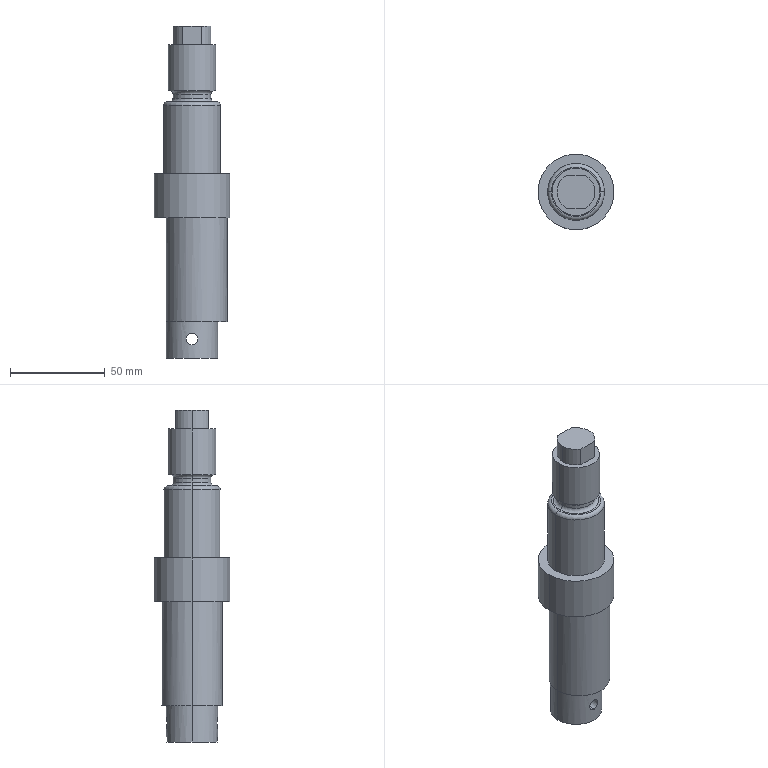Part | SolidWorks | features Boss 6, Chamfer 2, Cut 2, Extrusion 1, Fillet 1 | 1 solid | 33 faces | box 40 x 40 x 175 mm | volume 126777 mm3 | cylinder 17 | plane 10 | torus 6 | commonest cylinder face diameters 20 x5 6 x2 25 x2 27 x2 30 x2 32 x2
STEP:
#1=CARTESIAN_POINT('',(-12.,0.,141.));
#2=VERTEX_POINT('',#1);
#3=CARTESIAN_POINT('',(12.,0.,141.));
#4=VERTEX_POINT('',#3);
#5=CARTESIAN_POINT('',(0.,0.,141.));
#6=DIRECTION('',(0.,0.,1.));
#7=DIRECTION('',(1.,0.,0.));
#8=AXIS2_PLACEMENT_3D('',#5,#6,#7);
#9=CIRCLE('',#8,12.);
#10=EDGE_CURVE('',#2,#4,#9,.T.);
#11=ORIENTED_EDGE('',*,*,#10,.F.);
#12=CARTESIAN_POINT('',(-10.,0.,139.));
#13=VERTEX_POINT('',#12);
#14=CARTESIAN_POINT('',(-12.,0.,139.));
#15=DIRECTION('',(0.,1.,0.));
#16=DIRECTION('',(-1.,0.,0.));
#17=AXIS2_PLACEMENT_3D('',#14,#15,#16);
#18=CIRCLE('',#17,2.);
#19=EDGE_CURVE('',#2,#13,#18,.T.);
#20=ORIENTED_EDGE('',*,*,#19,.T.);
#21=CARTESIAN_POINT('',(10.,0.,139.));
#22=VERTEX_POINT('',#21);
#23=CARTESIAN_POINT('',(0.,0.,139.));
#24=DIRECTION('',(0.,0.,-1.));
#25=DIRECTION('',(1.,0.,0.));
#26=AXIS2_PLACEMENT_3D('',#23,#24,#25);
#27=CIRCLE('',#26,10.);
#28=EDGE_CURVE('',#22,#13,#27,.T.);
#29=ORIENTED_EDGE('',*,*,#28,.F.);
#30=CARTESIAN_POINT('',(12.,0.,139.));
#31=DIRECTION('',(0.,-1.,0.));
#32=DIRECTION('',(0.,0.,-1.));
#33=AXIS2_PLACEMENT_3D('',#30,#31,#32);
#34=CIRCLE('',#33,2.);
#35=EDGE_CURVE('',#4,#22,#34,.T.);
#36=ORIENTED_EDGE('',*,*,#35,.F.);
#37=EDGE_LOOP('',(#11,#20,#29,#36));
#38=FACE_OUTER_BOUND('',#37,.T.);
#39=CARTESIAN_POINT('',(0.,0.,139.));
#40=DIRECTION('',(0.,0.,1.));
#41=DIRECTION('',(1.,0.,0.));
#42=AXIS2_PLACEMENT_3D('',#39,#40,#41);
#43=TOROIDAL_SURFACE('',#42,12.,2.);
#44=ADVANCED_FACE('',(#38),#43,.F.);
#45=CARTESIAN_POINT('',(-15.,0.,133.));
#46=VERTEX_POINT('',#45);
#47=CARTESIAN_POINT('',(15.,0.,133.));
#48=VERTEX_POINT('',#47);
#49=CARTESIAN_POINT('',(0.,0.,133.));
#50=DIRECTION('',(0.,0.,-1.));
#51=DIRECTION('',(1.,0.,0.));
#52=AXIS2_PLACEMENT_3D('',#49,#50,#51);
#53=CIRCLE('',#52,15.);
#54=EDGE_CURVE('',#46,#48,#53,.T.);
#55=ORIENTED_EDGE('',*,*,#54,.F.);
#56=CARTESIAN_POINT('',(-13.,0.,135.));
#57=VERTEX_POINT('',#56);
#58=CARTESIAN_POINT('',(-13.,0.,133.));
#59=DIRECTION('',(0.,1.,0.));
#60=DIRECTION('',(-1.,0.,0.));
#61=AXIS2_PLACEMENT_3D('',#58,#59,#60);
#62=CIRCLE('',#61,2.);
#63=EDGE_CURVE('',#46,#57,#62,.T.);
#64=ORIENTED_EDGE('',*,*,#63,.T.);
#65=CARTESIAN_POINT('',(13.,0.,135.));
#66=VERTEX_POINT('',#65);
#67=CARTESIAN_POINT('',(0.,0.,135.));
#68=DIRECTION('',(0.,0.,1.));
#69=DIRECTION('',(1.,0.,0.));
#70=AXIS2_PLACEMENT_3D('',#67,#68,#69);
#71=CIRCLE('',#70,13.);
#72=EDGE_CURVE('',#66,#57,#71,.T.);
#73=ORIENTED_EDGE('',*,*,#72,.F.);
#74=CARTESIAN_POINT('',(13.,0.,133.));
#75=DIRECTION('',(0.,-1.,0.));
#76=DIRECTION('',(0.,0.,-1.));
#77=AXIS2_PLACEMENT_3D('',#74,#75,#76);
#78=CIRCLE('',#77,2.);
#79=EDGE_CURVE('',#48,#66,#78,.T.);
#80=ORIENTED_EDGE('',*,*,#79,.F.);
#81=EDGE_LOOP('',(#55,#64,#73,#80));
#82=FACE_OUTER_BOUND('',#81,.T.);
#83=CARTESIAN_POINT('',(0.,0.,133.));
#84=DIRECTION('',(0.,0.,1.));
#85=DIRECTION('',(1.,0.,0.));
#86=AXIS2_PLACEMENT_3D('',#83,#84,#85);
#87=TOROIDAL_SURFACE('',#86,13.,2.);
#88=ADVANCED_FACE('',(#82),#87,.T.);
#89=CARTESIAN_POINT('',(-10.,0.,137.));
#90=VERTEX_POINT('',#89);
#91=CARTESIAN_POINT('',(10.,0.,137.));
#92=VERTEX_POINT('',#91);
#93=CARTESIAN_POINT('',(0.,0.,137.));
#94=DIRECTION('',(0.,0.,1.));
#95=DIRECTION('',(1.,0.,0.));
#96=AXIS2_PLACEMENT_3D('',#93,#94,#95);
#97=CIRCLE('',#96,10.);
#98=EDGE_CURVE('',#90,#92,#97,.T.);
#99=ORIENTED_EDGE('',*,*,#98,.F.);
#100=CARTESIAN_POINT('',(-12.,0.,135.));
#101=VERTEX_POINT('',#100);
#102=CARTESIAN_POINT('',(-12.,0.,137.));
#103=DIRECTION('',(0.,1.,0.));
#104=DIRECTION('',(-1.,0.,0.));
#105=AXIS2_PLACEMENT_3D('',#102,#103,#104);
#106=CIRCLE('',#105,2.);
#107=EDGE_CURVE('',#90,#101,#106,.T.);
#108=ORIENTED_EDGE('',*,*,#107,.T.);
#109=CARTESIAN_POINT('',(12.,0.,135.));
#110=VERTEX_POINT('',#109);
#111=CARTESIAN_POINT('',(0.,0.,135.));
#112=DIRECTION('',(0.,0.,-1.));
#113=DIRECTION('',(1.,0.,0.));
#114=AXIS2_PLACEMENT_3D('',#111,#112,#113);
#115=CIRCLE('',#114,12.);
#116=EDGE_CURVE('',#110,#101,#115,.T.);
#117=ORIENTED_EDGE('',*,*,#116,.F.);
#118=CARTESIAN_POINT('',(12.,0.,137.));
#119=DIRECTION('',(0.,-1.,0.));
#120=DIRECTION('',(0.,0.,-1.));
#121=AXIS2_PLACEMENT_3D('',#118,#119,#120);
#122=CIRCLE('',#121,2.);
#123=EDGE_CURVE('',#92,#110,#122,.T.);
#124=ORIENTED_EDGE('',*,*,#123,.F.);
#125=EDGE_LOOP('',(#99,#108,#117,#124));
#126=FACE_OUTER_BOUND('',#125,.T.);
#127=CARTESIAN_POINT('',(0.,0.,137.));
#128=DIRECTION('',(0.,0.,1.));
#129=DIRECTION('',(1.,0.,0.));
#130=AXIS2_PLACEMENT_3D('',#127,#128,#129);
#131=TOROIDAL_SURFACE('',#130,12.,2.);
#132=ADVANCED_FACE('',(#126),#131,.F.);
#133=CARTESIAN_POINT('',(0.,-13.5,7.));
#134=VERTEX_POINT('',#133);
#135=CARTESIAN_POINT('',(0.,-13.5,13.));
#136=VERTEX_POINT('',#135);
#137=CARTESIAN_POINT('',(0.,-13.5,7.));
#138=CARTESIAN_POINT('',(-0.3922,-13.5,7.));
#139=CARTESIAN_POINT('',(-0.7881,-13.482,7.079));
#140=CARTESIAN_POINT('',(-1.33,-13.436,7.304));
#141=CARTESIAN_POINT('',(-1.505,-13.417,7.398));
#142=CARTESIAN_POINT('',(-1.831,-13.376,7.616));
#143=CARTESIAN_POINT('',(-1.982,-13.354,7.739));
#144=CARTESIAN_POINT('',(-2.259,-13.31,8.016));
#145=CARTESIAN_POINT('',(-2.385,-13.288,8.17));
#146=CARTESIAN_POINT('',(-2.602,-13.247,8.494));
#147=CARTESIAN_POINT('',(-2.694,-13.229,8.666));
#148=CARTESIAN_POINT('',(-2.922,-13.181,9.212));
#149=CARTESIAN_POINT('',(-3.,-13.162,9.603));
#150=CARTESIAN_POINT('',(-3.,-13.162,10.197));
#151=CARTESIAN_POINT('',(-2.981,-13.167,10.392));
#152=CARTESIAN_POINT('',(-2.904,-13.184,10.777));
#153=CARTESIAN_POINT('',(-2.846,-13.197,10.968));
#154=CARTESIAN_POINT('',(-2.696,-13.228,11.33));
#155=CARTESIAN_POINT('',(-2.604,-13.247,11.502));
#156=CARTESIAN_POINT('',(-2.386,-13.288,11.829));
#157=CARTESIAN_POINT('',(-2.26,-13.31,11.982));
#158=CARTESIAN_POINT('',(-1.985,-13.354,12.258));
#159=CARTESIAN_POINT('',(-1.834,-13.376,12.383));
#160=CARTESIAN_POINT('',(-1.506,-13.417,12.602));
#161=CARTESIAN_POINT('',(-1.333,-13.435,12.694));
#162=CARTESIAN_POINT('',(-0.9726,-13.466,12.845));
#163=CARTESIAN_POINT('',(-0.7819,-13.479,12.903));
#164=CARTESIAN_POINT('',(-0.395,-13.496,12.98));
#165=CARTESIAN_POINT('',(-0.1988,-13.5,13.));
#166=CARTESIAN_POINT('',(0.,-13.5,13.));
#167=B_SPLINE_CURVE_WITH_KNOTS('',3,(#137,#138,#139,#140,#141,#142,#143,#144,#145,#146,#147,#148,#149,#150,#151,#152,#153,#154,#155,#156,#157,#158,#159,#160,#161,#162,#163,#164,#165,#166),.UNSPECIFIED.,.F.,.F.,(4,2,2,2,2,2,2,2,2,2,2,2,2,2,4),(0.009409,0.01058,0.01117,0.01176,0.01235,0.01294,0.01411,0.0147,0.01529,0.01588,0.01646,0.01705,0.01764,0.01823,0.01882),.UNSPECIFIED.);
#168=EDGE_CURVE('',#134,#136,#167,.T.);
#169=ORIENTED_EDGE('',*,*,#168,.F.);
#170=CARTESIAN_POINT('',(0.,13.5,7.));
#171=VERTEX_POINT('',#170);
#172=CARTESIAN_POINT('',(0.,-15.,7.));
#173=DIRECTION('',(0.,1.,0.));
#174=VECTOR('',#173,1000.);
#175=LINE('',#172,#174);
#176=EDGE_CURVE('',#134,#171,#175,.T.);
#177=ORIENTED_EDGE('',*,*,#176,.T.);
#178=CARTESIAN_POINT('',(0.,13.5,13.));
#179=VERTEX_POINT('',#178);
#180=CARTESIAN_POINT('',(0.,13.5,13.));
#181=CARTESIAN_POINT('',(-0.1989,13.5,13.));
#182=CARTESIAN_POINT('',(-0.3943,13.496,12.98));
#183=CARTESIAN_POINT('',(-0.7786,13.479,12.904));
#184=CARTESIAN_POINT('',(-0.9695,13.466,12.846));
#185=CARTESIAN_POINT('',(-1.333,13.435,12.695));
#186=CARTESIAN_POINT('',(-1.505,13.417,12.603));
#187=CARTESIAN_POINT('',(-1.83,13.376,12.385));
#188=CARTESIAN_POINT('',(-1.984,13.354,12.259));
#189=CARTESIAN_POINT('',(-2.26,13.31,11.983));
#190=CARTESIAN_POINT('',(-2.384,13.288,11.832));
#191=CARTESIAN_POINT('',(-2.603,13.247,11.504));
#192=CARTESIAN_POINT('',(-2.696,13.228,11.331));
#193=CARTESIAN_POINT('',(-2.846,13.197,10.97));
#194=CARTESIAN_POINT('',(-2.903,13.184,10.78));
#195=CARTESIAN_POINT('',(-2.981,13.167,10.393));
#196=CARTESIAN_POINT('',(-3.,13.162,10.198));
#197=CARTESIAN_POINT('',(-3.,13.162,9.805));
#198=CARTESIAN_POINT('',(-2.98,13.167,9.605));
#199=CARTESIAN_POINT('',(-2.903,13.184,9.22));
#200=CARTESIAN_POINT('',(-2.847,13.197,9.033));
#201=CARTESIAN_POINT('',(-2.696,13.228,8.669));
#202=CARTESIAN_POINT('',(-2.602,13.247,8.494));
#203=CARTESIAN_POINT('',(-2.385,13.288,8.17));
#204=CARTESIAN_POINT('',(-2.26,13.31,8.018));
#205=CARTESIAN_POINT('',(-1.982,13.354,7.739));
#206=CARTESIAN_POINT('',(-1.831,13.376,7.616));
#207=CARTESIAN_POINT('',(-1.507,13.417,7.398));
#208=CARTESIAN_POINT('',(-1.331,13.435,7.304));
#209=CARTESIAN_POINT('',(-0.9683,13.466,7.154));
#210=CARTESIAN_POINT('',(-0.7813,13.479,7.097));
#211=CARTESIAN_POINT('',(-0.3953,13.496,7.02));
#212=CARTESIAN_POINT('',(-0.1961,13.5,7.));
#213=CARTESIAN_POINT('',(0.,13.5,7.));
#214=B_SPLINE_CURVE_WITH_KNOTS('',3,(#180,#181,#182,#183,#184,#185,#186,#187,#188,#189,#190,#191,#192,#193,#194,#195,#196,#197,#198,#199,#200,#201,#202,#203,#204,#205,#206,#207,#208,#209,#210,#211,#212,#213),.UNSPECIFIED.,.F.,.F.,(4,2,2,2,2,2,2,2,2,2,2,2,2,2,2,2,4),(0.,0.0005881,0.001176,0.001764,0.002352,0.00294,0.003528,0.004116,0.004704,0.005292,0.005881,0.006469,0.007057,0.007645,0.008233,0.008821,0.009409),.UNSPECIFIED.);
#215=EDGE_CURVE('',#179,#171,#214,.T.);
#216=ORIENTED_EDGE('',*,*,#215,.F.);
#217=CARTESIAN_POINT('',(0.,-15.,13.));
#218=DIRECTION('',(0.,1.,0.));
#219=VECTOR('',#218,1000.);
#220=LINE('',#217,#219);
#221=EDGE_CURVE('',#136,#179,#220,.T.);
#222=ORIENTED_EDGE('',*,*,#221,.F.);
#223=EDGE_LOOP('',(#169,#177,#216,#222));
#224=FACE_OUTER_BOUND('',#223,.T.);
#225=CARTESIAN_POINT('',(0.,-15.,10.));
#226=DIRECTION('',(0.,1.,0.));
#227=DIRECTION('',(0.,0.,1.));
#228=AXIS2_PLACEMENT_3D('',#225,#226,#227);
#229=CYLINDRICAL_SURFACE('',#228,3.);
#230=ADVANCED_FACE('',(#224),#229,.F.);
#231=CARTESIAN_POINT('',(-10.,0.,175.));
#232=VERTEX_POINT('',#231);
#233=CARTESIAN_POINT('',(-5.,-8.66,175.));
#234=VERTEX_POINT('',#233);
#235=CARTESIAN_POINT('',(0.,0.,175.));
#236=DIRECTION('',(0.,0.,1.));
#237=DIRECTION('',(1.,0.,0.));
#238=AXIS2_PLACEMENT_3D('',#235,#236,#237);
#239=CIRCLE('',#238,10.);
#240=EDGE_CURVE('',#232,#234,#239,.T.);
#241=ORIENTED_EDGE('',*,*,#240,.F.);
#242=CARTESIAN_POINT('',(-10.,0.,165.));
#243=VERTEX_POINT('',#242);
#244=CARTESIAN_POINT('',(-10.,0.,175.));
#245=DIRECTION('',(0.,0.,-1.));
#246=VECTOR('',#245,1000.);
#247=LINE('',#244,#246);
#248=EDGE_CURVE('',#232,#243,#247,.T.);
#249=ORIENTED_EDGE('',*,*,#248,.T.);
#250=CARTESIAN_POINT('',(-5.,-8.66,165.));
#251=VERTEX_POINT('',#250);
#252=CARTESIAN_POINT('',(0.,0.,165.));
#253=DIRECTION('',(0.,0.,1.));
#254=DIRECTION('',(1.,0.,0.));
#255=AXIS2_PLACEMENT_3D('',#252,#253,#254);
#256=CIRCLE('',#255,10.);
#257=EDGE_CURVE('',#243,#251,#256,.T.);
#258=ORIENTED_EDGE('',*,*,#257,.T.);
#259=CARTESIAN_POINT('',(-5.,-8.66,175.));
#260=DIRECTION('',(0.,0.,-1.));
#261=VECTOR('',#260,1000.);
#262=LINE('',#259,#261);
#263=EDGE_CURVE('',#234,#251,#262,.T.);
#264=ORIENTED_EDGE('',*,*,#263,.F.);
#265=EDGE_LOOP('',(#241,#249,#258,#264));
#266=FACE_OUTER_BOUND('',#265,.T.);
#267=CARTESIAN_POINT('',(0.,0.,175.));
#268=DIRECTION('',(0.,0.,-1.));
#269=DIRECTION('',(-1.,0.,0.));
#270=AXIS2_PLACEMENT_3D('',#267,#268,#269);
#271=CYLINDRICAL_SURFACE('',#270,10.);
#272=ADVANCED_FACE('',(#266),#271,.T.);
#273=CARTESIAN_POINT('',(12.5,0.,165.));
#274=VERTEX_POINT('',#273);
#275=CARTESIAN_POINT('',(-12.5,0.,165.));
#276=VERTEX_POINT('',#275);
#277=CARTESIAN_POINT('',(0.,0.,165.));
#278=DIRECTION('',(0.,0.,1.));
#279=DIRECTION('',(1.,0.,0.));
#280=AXIS2_PLACEMENT_3D('',#277,#278,#279);
#281=CIRCLE('',#280,12.5);
#282=EDGE_CURVE('',#274,#276,#281,.T.);
#283=ORIENTED_EDGE('',*,*,#282,.F.);
#284=CARTESIAN_POINT('',(12.5,0.,141.));
#285=VERTEX_POINT('',#284);
#286=CARTESIAN_POINT('',(12.5,0.,165.));
#287=DIRECTION('',(0.,0.,-1.));
#288=VECTOR('',#287,1000.);
#289=LINE('',#286,#288);
#290=EDGE_CURVE('',#274,#285,#289,.T.);
#291=ORIENTED_EDGE('',*,*,#290,.T.);
#292=CARTESIAN_POINT('',(-12.5,0.,141.));
#293=VERTEX_POINT('',#292);
#294=CARTESIAN_POINT('',(0.,0.,141.));
#295=DIRECTION('',(0.,0.,1.));
#296=DIRECTION('',(1.,0.,0.));
#297=AXIS2_PLACEMENT_3D('',#294,#295,#296);
#298=CIRCLE('',#297,12.5);
#299=EDGE_CURVE('',#285,#293,#298,.T.);
#300=ORIENTED_EDGE('',*,*,#299,.T.);
#301=CARTESIAN_POINT('',(-12.5,0.,165.));
#302=DIRECTION('',(0.,0.,-1.));
#303=VECTOR('',#302,1000.);
#304=LINE('',#301,#303);
#305=EDGE_CURVE('',#276,#293,#304,.T.);
#306=ORIENTED_EDGE('',*,*,#305,.F.);
#307=EDGE_LOOP('',(#283,#291,#300,#306));
#308=FACE_OUTER_BOUND('',#307,.T.);
#309=CARTESIAN_POINT('',(0.,0.,165.));
#310=DIRECTION('',(0.,0.,-1.));
#311=DIRECTION('',(-1.,0.,0.));
#312=AXIS2_PLACEMENT_3D('',#309,#310,#311);
#313=CYLINDRICAL_SURFACE('',#312,12.5);
#314=ADVANCED_FACE('',(#308),#313,.T.);
#315=CARTESIAN_POINT('',(0.,0.,139.));
#316=DIRECTION('',(0.,0.,-1.));
#317=DIRECTION('',(1.,0.,0.));
#318=AXIS2_PLACEMENT_3D('',#315,#316,#317);
#319=CIRCLE('',#318,10.);
#320=EDGE_CURVE('',#13,#22,#319,.T.);
#321=ORIENTED_EDGE('',*,*,#320,.T.);
#322=CARTESIAN_POINT('',(10.,0.,141.));
#323=DIRECTION('',(0.,0.,-1.));
#324=VECTOR('',#323,1000.);
#325=LINE('',#322,#324);
#326=EDGE_CURVE('',#22,#92,#325,.T.);
#327=ORIENTED_EDGE('',*,*,#326,.T.);
#328=CARTESIAN_POINT('',(0.,0.,137.));
#329=DIRECTION('',(0.,0.,1.));
#330=DIRECTION('',(1.,0.,0.));
#331=AXIS2_PLACEMENT_3D('',#328,#329,#330);
#332=CIRCLE('',#331,10.);
#333=EDGE_CURVE('',#92,#90,#332,.T.);
#334=ORIENTED_EDGE('',*,*,#333,.T.);
#335=CARTESIAN_POINT('',(-10.,0.,141.));
#336=DIRECTION('',(0.,0.,-1.));
#337=VECTOR('',#336,1000.);
#338=LINE('',#335,#337);
#339=EDGE_CURVE('',#13,#90,#338,.T.);
#340=ORIENTED_EDGE('',*,*,#339,.F.);
#341=EDGE_LOOP('',(#321,#327,#334,#340));
#342=FACE_OUTER_BOUND('',#341,.T.);
#343=CARTESIAN_POINT('',(0.,0.,141.));
#344=DIRECTION('',(0.,0.,-1.));
#345=DIRECTION('',(-1.,0.,0.));
#346=AXIS2_PLACEMENT_3D('',#343,#344,#345);
#347=CYLINDRICAL_SURFACE('',#346,10.);
#348=ADVANCED_FACE('',(#342),#347,.T.);
#349=ORIENTED_EDGE('',*,*,#54,.T.);
#350=CARTESIAN_POINT('',(15.,0.,97.));
#351=VERTEX_POINT('',#350);
#352=CARTESIAN_POINT('',(15.,0.,135.));
#353=DIRECTION('',(0.,0.,-1.));
#354=VECTOR('',#353,1000.);
#355=LINE('',#352,#354);
#356=EDGE_CURVE('',#48,#351,#355,.T.);
#357=ORIENTED_EDGE('',*,*,#356,.T.);
#358=CARTESIAN_POINT('',(-15.,0.,97.));
#359=VERTEX_POINT('',#358);
#360=CARTESIAN_POINT('',(0.,0.,97.));
#361=DIRECTION('',(0.,0.,1.));
#362=DIRECTION('',(1.,0.,0.));
#363=AXIS2_PLACEMENT_3D('',#360,#361,#362);
#364=CIRCLE('',#363,15.);
#365=EDGE_CURVE('',#351,#359,#364,.T.);
#366=ORIENTED_EDGE('',*,*,#365,.T.);
#367=CARTESIAN_POINT('',(-15.,0.,135.));
#368=DIRECTION('',(0.,0.,-1.));
#369=VECTOR('',#368,1000.);
#370=LINE('',#367,#369);
#371=EDGE_CURVE('',#46,#359,#370,.T.);
#372=ORIENTED_EDGE('',*,*,#371,.F.);
#373=EDGE_LOOP('',(#349,#357,#366,#372));
#374=FACE_OUTER_BOUND('',#373,.T.);
#375=CARTESIAN_POINT('',(0.,0.,135.));
#376=DIRECTION('',(0.,0.,-1.));
#377=DIRECTION('',(-1.,0.,0.));
#378=AXIS2_PLACEMENT_3D('',#375,#376,#377);
#379=CYLINDRICAL_SURFACE('',#378,15.);
#380=ADVANCED_FACE('',(#374),#379,.T.);
#381=CARTESIAN_POINT('',(20.,0.,97.));
#382=VERTEX_POINT('',#381);
#383=CARTESIAN_POINT('',(-20.,0.,97.));
#384=VERTEX_POINT('',#383);
#385=CARTESIAN_POINT('',(0.,0.,97.));
#386=DIRECTION('',(0.,0.,1.));
#387=DIRECTION('',(1.,0.,0.));
#388=AXIS2_PLACEMENT_3D('',#385,#386,#387);
#389=CIRCLE('',#388,20.);
#390=EDGE_CURVE('',#382,#384,#389,.T.);
#391=ORIENTED_EDGE('',*,*,#390,.F.);
#392=CARTESIAN_POINT('',(20.,0.,74.));
#393=VERTEX_POINT('',#392);
#394=CARTESIAN_POINT('',(20.,0.,97.));
#395=DIRECTION('',(0.,0.,-1.));
#396=VECTOR('',#395,1000.);
#397=LINE('',#394,#396);
#398=EDGE_CURVE('',#382,#393,#397,.T.);
#399=ORIENTED_EDGE('',*,*,#398,.T.);
#400=CARTESIAN_POINT('',(-20.,0.,74.));
#401=VERTEX_POINT('',#400);
#402=CARTESIAN_POINT('',(0.,0.,74.));
#403=DIRECTION('',(0.,0.,1.));
#404=DIRECTION('',(1.,0.,0.));
#405=AXIS2_PLACEMENT_3D('',#402,#403,#404);
#406=CIRCLE('',#405,20.);
#407=EDGE_CURVE('',#393,#401,#406,.T.);
#408=ORIENTED_EDGE('',*,*,#407,.T.);
#409=CARTESIAN_POINT('',(-20.,0.,97.));
#410=DIRECTION('',(0.,0.,-1.));
#411=VECTOR('',#410,1000.);
#412=LINE('',#409,#411);
#413=EDGE_CURVE('',#384,#401,#412,.T.);
#414=ORIENTED_EDGE('',*,*,#413,.F.);
#415=EDGE_LOOP('',(#391,#399,#408,#414));
#416=FACE_OUTER_BOUND('',#415,.T.);
#417=CARTESIAN_POINT('',(0.,0.,97.));
#418=DIRECTION('',(0.,0.,-1.));
#419=DIRECTION('',(-1.,0.,0.));
#420=AXIS2_PLACEMENT_3D('',#417,#418,#419);
#421=CYLINDRICAL_SURFACE('',#420,20.);
#422=ADVANCED_FACE('',(#416),#421,.T.);
#423=CARTESIAN_POINT('',(18.5,0.,74.));
#424=VERTEX_POINT('',#423);
#425=CARTESIAN_POINT('',(-13.5,0.,74.));
#426=VERTEX_POINT('',#425);
#427=CARTESIAN_POINT('',(2.5,0.,74.));
#428=DIRECTION('',(0.,0.,1.));
#429=DIRECTION('',(1.,0.,0.));
#430=AXIS2_PLACEMENT_3D('',#427,#428,#429);
#431=CIRCLE('',#430,16.);
#432=EDGE_CURVE('',#424,#426,#431,.T.);
#433=ORIENTED_EDGE('',*,*,#432,.F.);
#434=CARTESIAN_POINT('',(18.5,0.,19.));
#435=VERTEX_POINT('',#434);
#436=CARTESIAN_POINT('',(18.5,0.,74.));
#437=DIRECTION('',(0.,0.,-1.));
#438=VECTOR('',#437,1000.);
#439=LINE('',#436,#438);
#440=EDGE_CURVE('',#424,#435,#439,.T.);
#441=ORIENTED_EDGE('',*,*,#440,.T.);
#442=CARTESIAN_POINT('',(-13.5,0.,19.));
#443=VERTEX_POINT('',#442);
#444=CARTESIAN_POINT('',(2.5,0.,19.));
#445=DIRECTION('',(0.,0.,1.));
#446=DIRECTION('',(1.,0.,0.));
#447=AXIS2_PLACEMENT_3D('',#444,#445,#446);
#448=CIRCLE('',#447,16.);
#449=EDGE_CURVE('',#435,#443,#448,.T.);
#450=ORIENTED_EDGE('',*,*,#449,.T.);
#451=CARTESIAN_POINT('',(-13.5,0.,74.));
#452=DIRECTION('',(0.,0.,-1.));
#453=VECTOR('',#452,1000.);
#454=LINE('',#451,#453);
#455=EDGE_CURVE('',#426,#443,#454,.T.);
#456=ORIENTED_EDGE('',*,*,#455,.F.);
#457=EDGE_LOOP('',(#433,#441,#450,#456));
#458=FACE_OUTER_BOUND('',#457,.T.);
#459=CARTESIAN_POINT('',(2.5,0.,74.));
#460=DIRECTION('',(0.,0.,-1.));
#461=DIRECTION('',(-1.,0.,0.));
#462=AXIS2_PLACEMENT_3D('',#459,#460,#461);
#463=CYLINDRICAL_SURFACE('',#462,16.);
#464=ADVANCED_FACE('',(#458),#463,.T.);
#465=ORIENTED_EDGE('',*,*,#215,.T.);
#466=CARTESIAN_POINT('',(0.,13.5,7.));
#467=CARTESIAN_POINT('',(0.3922,13.5,7.));
#468=CARTESIAN_POINT('',(0.7881,13.482,7.079));
#469=CARTESIAN_POINT('',(1.33,13.436,7.304));
#470=CARTESIAN_POINT('',(1.505,13.417,7.398));
#471=CARTESIAN_POINT('',(1.831,13.376,7.616));
#472=CARTESIAN_POINT('',(1.982,13.354,7.739));
#473=CARTESIAN_POINT('',(2.259,13.31,8.016));
#474=CARTESIAN_POINT('',(2.385,13.288,8.17));
#475=CARTESIAN_POINT('',(2.602,13.247,8.494));
#476=CARTESIAN_POINT('',(2.694,13.229,8.666));
#477=CARTESIAN_POINT('',(2.922,13.181,9.212));
#478=CARTESIAN_POINT('',(3.,13.162,9.603));
#479=CARTESIAN_POINT('',(3.,13.162,10.197));
#480=CARTESIAN_POINT('',(2.981,13.167,10.392));
#481=CARTESIAN_POINT('',(2.904,13.184,10.777));
#482=CARTESIAN_POINT('',(2.846,13.197,10.968));
#483=CARTESIAN_POINT('',(2.696,13.228,11.33));
#484=CARTESIAN_POINT('',(2.604,13.247,11.502));
#485=CARTESIAN_POINT('',(2.386,13.288,11.829));
#486=CARTESIAN_POINT('',(2.26,13.31,11.982));
#487=CARTESIAN_POINT('',(1.985,13.354,12.258));
#488=CARTESIAN_POINT('',(1.834,13.376,12.383));
#489=CARTESIAN_POINT('',(1.506,13.417,12.602));
#490=CARTESIAN_POINT('',(1.333,13.435,12.694));
#491=CARTESIAN_POINT('',(0.9726,13.466,12.845));
#492=CARTESIAN_POINT('',(0.7819,13.479,12.903));
#493=CARTESIAN_POINT('',(0.395,13.496,12.98));
#494=CARTESIAN_POINT('',(0.1988,13.5,13.));
#495=CARTESIAN_POINT('',(0.,13.5,13.));
#496=B_SPLINE_CURVE_WITH_KNOTS('',3,(#466,#467,#468,#469,#470,#471,#472,#473,#474,#475,#476,#477,#478,#479,#480,#481,#482,#483,#484,#485,#486,#487,#488,#489,#490,#491,#492,#493,#494,#495),.UNSPECIFIED.,.F.,.F.,(4,2,2,2,2,2,2,2,2,2,2,2,2,2,4),(0.009409,0.01058,0.01117,0.01176,0.01235,0.01294,0.01411,0.0147,0.01529,0.01588,0.01646,0.01705,0.01764,0.01823,0.01882),.UNSPECIFIED.);
#497=EDGE_CURVE('',#171,#179,#496,.T.);
#498=ORIENTED_EDGE('',*,*,#497,.T.);
#499=EDGE_LOOP('',(#465,#498));
#500=FACE_BOUND('',#499,.T.);
#501=CARTESIAN_POINT('',(13.5,0.,19.));
#502=VERTEX_POINT('',#501);
#503=CARTESIAN_POINT('',(0.,0.,19.));
#504=DIRECTION('',(0.,0.,1.));
#505=DIRECTION('',(1.,0.,0.));
#506=AXIS2_PLACEMENT_3D('',#503,#504,#505);
#507=CIRCLE('',#506,13.5);
#508=EDGE_CURVE('',#502,#443,#507,.T.);
#509=ORIENTED_EDGE('',*,*,#508,.F.);
#510=CARTESIAN_POINT('',(13.5,0.,0.));
#511=VERTEX_POINT('',#510);
#512=CARTESIAN_POINT('',(13.5,0.,19.));
#513=DIRECTION('',(0.,0.,-1.));
#514=VECTOR('',#513,1000.);
#515=LINE('',#512,#514);
#516=EDGE_CURVE('',#502,#511,#515,.T.);
#517=ORIENTED_EDGE('',*,*,#516,.T.);
#518=CARTESIAN_POINT('',(-13.5,0.,0.));
#519=VERTEX_POINT('',#518);
#520=CARTESIAN_POINT('',(0.,0.,0.));
#521=DIRECTION('',(0.,0.,1.));
#522=DIRECTION('',(1.,0.,0.));
#523=AXIS2_PLACEMENT_3D('',#520,#521,#522);
#524=CIRCLE('',#523,13.5);
#525=EDGE_CURVE('',#511,#519,#524,.T.);
#526=ORIENTED_EDGE('',*,*,#525,.T.);
#527=CARTESIAN_POINT('',(-13.5,0.,19.));
#528=DIRECTION('',(0.,0.,-1.));
#529=VECTOR('',#528,1000.);
#530=LINE('',#527,#529);
#531=EDGE_CURVE('',#443,#519,#530,.T.);
#532=ORIENTED_EDGE('',*,*,#531,.F.);
#533=EDGE_LOOP('',(#509,#517,#526,#532));
#534=FACE_OUTER_BOUND('',#533,.T.);
#535=CARTESIAN_POINT('',(0.,0.,19.));
#536=DIRECTION('',(0.,0.,-1.));
#537=DIRECTION('',(-1.,0.,0.));
#538=AXIS2_PLACEMENT_3D('',#535,#536,#537);
#539=CYLINDRICAL_SURFACE('',#538,13.5);
#540=ADVANCED_FACE('',(#500,#534),#539,.T.);
#541=CARTESIAN_POINT('',(0.,0.,165.));
#542=DIRECTION('',(0.,0.,1.));
#543=DIRECTION('',(1.,0.,0.));
#544=AXIS2_PLACEMENT_3D('',#541,#542,#543);
#545=CIRCLE('',#544,12.5);
#546=EDGE_CURVE('',#276,#274,#545,.T.);
#547=ORIENTED_EDGE('',*,*,#546,.T.);
#548=ORIENTED_EDGE('',*,*,#282,.T.);
#549=EDGE_LOOP('',(#547,#548));
#550=FACE_OUTER_BOUND('',#549,.T.);
#551=CARTESIAN_POINT('',(5.,-8.66,165.));
#552=VERTEX_POINT('',#551);
#553=CARTESIAN_POINT('',(-5.,-8.66,165.));
#554=DIRECTION('',(1.,0.,0.));
#555=VECTOR('',#554,1000.);
#556=LINE('',#553,#555);
#557=EDGE_CURVE('',#251,#552,#556,.T.);
#558=ORIENTED_EDGE('',*,*,#557,.F.);
#559=ORIENTED_EDGE('',*,*,#257,.F.);
#560=CARTESIAN_POINT('',(-5.,8.66,165.));
#561=VERTEX_POINT('',#560);
#562=CARTESIAN_POINT('',(0.,0.,165.));
#563=DIRECTION('',(0.,0.,1.));
#564=DIRECTION('',(1.,0.,0.));
#565=AXIS2_PLACEMENT_3D('',#562,#563,#564);
#566=CIRCLE('',#565,10.);
#567=EDGE_CURVE('',#561,#243,#566,.T.);
#568=ORIENTED_EDGE('',*,*,#567,.F.);
#569=CARTESIAN_POINT('',(5.,8.66,165.));
#570=VERTEX_POINT('',#569);
#571=CARTESIAN_POINT('',(-5.,8.66,165.));
#572=DIRECTION('',(-1.,0.,0.));
#573=VECTOR('',#572,1000.);
#574=LINE('',#571,#573);
#575=EDGE_CURVE('',#570,#561,#574,.T.);
#576=ORIENTED_EDGE('',*,*,#575,.F.);
#577=CARTESIAN_POINT('',(0.,0.,165.));
#578=DIRECTION('',(0.,0.,1.));
#579=DIRECTION('',(1.,0.,0.));
#580=AXIS2_PLACEMENT_3D('',#577,#578,#579);
#581=CIRCLE('',#580,10.);
#582=EDGE_CURVE('',#552,#570,#581,.T.);
#583=ORIENTED_EDGE('',*,*,#582,.F.);
#584=EDGE_LOOP('',(#558,#559,#568,#576,#583));
#585=FACE_BOUND('',#584,.T.);
#586=CARTESIAN_POINT('',(0.,0.,165.));
#587=DIRECTION('',(0.,0.,1.));
#588=DIRECTION('',(1.,0.,0.));
#589=AXIS2_PLACEMENT_3D('',#586,#587,#588);
#590=PLANE('',#589);
#591=ADVANCED_FACE('',(#550,#585),#590,.T.);
#592=ORIENTED_EDGE('',*,*,#116,.T.);
#593=CARTESIAN_POINT('',(0.,0.,135.));
#594=DIRECTION('',(0.,0.,-1.));
#595=DIRECTION('',(1.,0.,0.));
#596=AXIS2_PLACEMENT_3D('',#593,#594,#595);
#597=CIRCLE('',#596,12.);
#598=EDGE_CURVE('',#101,#110,#597,.T.);
#599=ORIENTED_EDGE('',*,*,#598,.T.);
#600=EDGE_LOOP('',(#592,#599));
#601=FACE_BOUND('',#600,.T.);
#602=ORIENTED_EDGE('',*,*,#72,.T.);
#603=CARTESIAN_POINT('',(0.,0.,135.));
#604=DIRECTION('',(0.,0.,1.));
#605=DIRECTION('',(1.,0.,0.));
#606=AXIS2_PLACEMENT_3D('',#603,#604,#605);
#607=CIRCLE('',#606,13.);
#608=EDGE_CURVE('',#57,#66,#607,.T.);
#609=ORIENTED_EDGE('',*,*,#608,.T.);
#610=EDGE_LOOP('',(#602,#609));
#611=FACE_OUTER_BOUND('',#610,.T.);
#612=CARTESIAN_POINT('',(0.,0.,135.));
#613=DIRECTION('',(0.,0.,1.));
#614=DIRECTION('',(1.,0.,0.));
#615=AXIS2_PLACEMENT_3D('',#612,#613,#614);
#616=PLANE('',#615);
#617=ADVANCED_FACE('',(#601,#611),#616,.T.);
#618=CARTESIAN_POINT('',(0.,0.,97.));
#619=DIRECTION('',(0.,0.,1.));
#620=DIRECTION('',(1.,0.,0.));
#621=AXIS2_PLACEMENT_3D('',#618,#619,#620);
#622=CIRCLE('',#621,20.);
#623=EDGE_CURVE('',#384,#382,#622,.T.);
#624=ORIENTED_EDGE('',*,*,#623,.T.);
#625=ORIENTED_EDGE('',*,*,#390,.T.);
#626=EDGE_LOOP('',(#624,#625));
#627=FACE_OUTER_BOUND('',#626,.T.);
#628=CARTESIAN_POINT('',(0.,0.,97.));
#629=DIRECTION('',(0.,0.,1.));
#630=DIRECTION('',(1.,0.,0.));
#631=AXIS2_PLACEMENT_3D('',#628,#629,#630);
#632=CIRCLE('',#631,15.);
#633=EDGE_CURVE('',#359,#351,#632,.T.);
#634=ORIENTED_EDGE('',*,*,#633,.F.);
#635=ORIENTED_EDGE('',*,*,#365,.F.);
#636=EDGE_LOOP('',(#634,#635));
#637=FACE_BOUND('',#636,.T.);
#638=CARTESIAN_POINT('',(0.,0.,97.));
#639=DIRECTION('',(0.,0.,1.));
#640=DIRECTION('',(1.,0.,0.));
#641=AXIS2_PLACEMENT_3D('',#638,#639,#640);
#642=PLANE('',#641);
#643=ADVANCED_FACE('',(#627,#637),#642,.T.);
#644=ORIENTED_EDGE('',*,*,#516,.F.);
#645=CARTESIAN_POINT('',(0.,0.,19.));
#646=DIRECTION('',(0.,0.,1.));
#647=DIRECTION('',(1.,0.,0.));
#648=AXIS2_PLACEMENT_3D('',#645,#646,#647);
#649=CIRCLE('',#648,13.5);
#650=EDGE_CURVE('',#443,#502,#649,.T.);
#651=ORIENTED_EDGE('',*,*,#650,.F.);
#652=ORIENTED_EDGE('',*,*,#531,.T.);
#653=CARTESIAN_POINT('',(0.,0.,0.));
#654=DIRECTION('',(0.,0.,1.));
#655=DIRECTION('',(1.,0.,0.));
#656=AXIS2_PLACEMENT_3D('',#653,#654,#655);
#657=CIRCLE('',#656,13.5);
#658=EDGE_CURVE('',#519,#511,#657,.T.);
#659=ORIENTED_EDGE('',*,*,#658,.T.);
#660=EDGE_LOOP('',(#644,#651,#652,#659));
#661=FACE_OUTER_BOUND('',#660,.T.);
#662=CARTESIAN_POINT('',(0.,-13.5,13.));
#663=CARTESIAN_POINT('',(0.1989,-13.5,13.));
#664=CARTESIAN_POINT('',(0.3943,-13.496,12.98));
#665=CARTESIAN_POINT('',(0.7786,-13.479,12.904));
#666=CARTESIAN_POINT('',(0.9695,-13.466,12.846));
#667=CARTESIAN_POINT('',(1.333,-13.435,12.695));
#668=CARTESIAN_POINT('',(1.505,-13.417,12.603));
#669=CARTESIAN_POINT('',(1.83,-13.376,12.385));
#670=CARTESIAN_POINT('',(1.984,-13.354,12.259));
#671=CARTESIAN_POINT('',(2.26,-13.31,11.983));
#672=CARTESIAN_POINT('',(2.384,-13.288,11.832));
#673=CARTESIAN_POINT('',(2.603,-13.247,11.504));
#674=CARTESIAN_POINT('',(2.696,-13.228,11.331));
#675=CARTESIAN_POINT('',(2.846,-13.197,10.97));
#676=CARTESIAN_POINT('',(2.903,-13.184,10.78));
#677=CARTESIAN_POINT('',(2.981,-13.167,10.393));
#678=CARTESIAN_POINT('',(3.,-13.162,10.198));
#679=CARTESIAN_POINT('',(3.,-13.162,9.805));
#680=CARTESIAN_POINT('',(2.98,-13.167,9.605));
#681=CARTESIAN_POINT('',(2.903,-13.184,9.22));
#682=CARTESIAN_POINT('',(2.847,-13.197,9.033));
#683=CARTESIAN_POINT('',(2.696,-13.228,8.669));
#684=CARTESIAN_POINT('',(2.602,-13.247,8.494));
#685=CARTESIAN_POINT('',(2.385,-13.288,8.17));
#686=CARTESIAN_POINT('',(2.26,-13.31,8.018));
#687=CARTESIAN_POINT('',(1.982,-13.354,7.739));
#688=CARTESIAN_POINT('',(1.831,-13.376,7.616));
#689=CARTESIAN_POINT('',(1.507,-13.417,7.398));
#690=CARTESIAN_POINT('',(1.331,-13.435,7.304));
#691=CARTESIAN_POINT('',(0.9683,-13.466,7.154));
#692=CARTESIAN_POINT('',(0.7813,-13.479,7.097));
#693=CARTESIAN_POINT('',(0.3953,-13.496,7.02));
#694=CARTESIAN_POINT('',(0.1961,-13.5,7.));
#695=CARTESIAN_POINT('',(0.,-13.5,7.));
#696=B_SPLINE_CURVE_WITH_KNOTS('',3,(#662,#663,#664,#665,#666,#667,#668,#669,#670,#671,#672,#673,#674,#675,#676,#677,#678,#679,#680,#681,#682,#683,#684,#685,#686,#687,#688,#689,#690,#691,#692,#693,#694,#695),.UNSPECIFIED.,.F.,.F.,(4,2,2,2,2,2,2,2,2,2,2,2,2,2,2,2,4),(0.,0.0005881,0.001176,0.001764,0.002352,0.00294,0.003528,0.004116,0.004704,0.005292,0.005881,0.006469,0.007057,0.007645,0.008233,0.008821,0.009409),.UNSPECIFIED.);
#697=EDGE_CURVE('',#136,#134,#696,.T.);
#698=ORIENTED_EDGE('',*,*,#697,.T.);
#699=ORIENTED_EDGE('',*,*,#168,.T.);
#700=EDGE_LOOP('',(#698,#699));
#701=FACE_BOUND('',#700,.T.);
#702=CARTESIAN_POINT('',(0.,0.,19.));
#703=DIRECTION('',(0.,0.,-1.));
#704=DIRECTION('',(-1.,0.,0.));
#705=AXIS2_PLACEMENT_3D('',#702,#703,#704);
#706=CYLINDRICAL_SURFACE('',#705,13.5);
#707=ADVANCED_FACE('',(#661,#701),#706,.T.);
#708=ORIENTED_EDGE('',*,*,#658,.F.);
#709=ORIENTED_EDGE('',*,*,#525,.F.);
#710=EDGE_LOOP('',(#708,#709));
#711=FACE_OUTER_BOUND('',#710,.T.);
#712=CARTESIAN_POINT('',(0.,0.,0.));
#713=DIRECTION('',(0.,0.,1.));
#714=DIRECTION('',(1.,0.,0.));
#715=AXIS2_PLACEMENT_3D('',#712,#713,#714);
#716=PLANE('',#715);
#717=ADVANCED_FACE('',(#711),#716,.F.);
#718=CARTESIAN_POINT('',(2.5,0.,19.));
#719=DIRECTION('',(0.,0.,1.));
#720=DIRECTION('',(1.,0.,0.));
#721=AXIS2_PLACEMENT_3D('',#718,#719,#720);
#722=CIRCLE('',#721,16.);
#723=EDGE_CURVE('',#443,#435,#722,.T.);
#724=ORIENTED_EDGE('',*,*,#723,.F.);
#725=ORIENTED_EDGE('',*,*,#650,.T.);
#726=ORIENTED_EDGE('',*,*,#508,.T.);
#727=ORIENTED_EDGE('',*,*,#449,.F.);
#728=EDGE_LOOP('',(#724,#725,#726,#727));
#729=FACE_OUTER_BOUND('',#728,.T.);
#730=CARTESIAN_POINT('',(2.5,0.,19.));
#731=DIRECTION('',(0.,0.,1.));
#732=DIRECTION('',(1.,0.,0.));
#733=AXIS2_PLACEMENT_3D('',#730,#731,#732);
#734=PLANE('',#733);
#735=ADVANCED_FACE('',(#729),#734,.F.);
#736=ORIENTED_EDGE('',*,*,#440,.F.);
#737=CARTESIAN_POINT('',(2.5,0.,74.));
#738=DIRECTION('',(0.,0.,1.));
#739=DIRECTION('',(1.,0.,0.));
#740=AXIS2_PLACEMENT_3D('',#737,#738,#739);
#741=CIRCLE('',#740,16.);
#742=EDGE_CURVE('',#426,#424,#741,.T.);
#743=ORIENTED_EDGE('',*,*,#742,.F.);
#744=ORIENTED_EDGE('',*,*,#455,.T.);
#745=ORIENTED_EDGE('',*,*,#723,.T.);
#746=EDGE_LOOP('',(#736,#743,#744,#745));
#747=FACE_OUTER_BOUND('',#746,.T.);
#748=CARTESIAN_POINT('',(2.5,0.,74.));
#749=DIRECTION('',(0.,0.,-1.));
#750=DIRECTION('',(-1.,0.,0.));
#751=AXIS2_PLACEMENT_3D('',#748,#749,#750);
#752=CYLINDRICAL_SURFACE('',#751,16.);
#753=ADVANCED_FACE('',(#747),#752,.T.);
#754=CARTESIAN_POINT('',(0.,0.,74.));
#755=DIRECTION('',(0.,0.,1.));
#756=DIRECTION('',(1.,0.,0.));
#757=AXIS2_PLACEMENT_3D('',#754,#755,#756);
#758=CIRCLE('',#757,20.);
#759=EDGE_CURVE('',#401,#393,#758,.T.);
#760=ORIENTED_EDGE('',*,*,#759,.F.);
#761=ORIENTED_EDGE('',*,*,#407,.F.);
#762=EDGE_LOOP('',(#760,#761));
#763=FACE_OUTER_BOUND('',#762,.T.);
#764=ORIENTED_EDGE('',*,*,#742,.T.);
#765=ORIENTED_EDGE('',*,*,#432,.T.);
#766=EDGE_LOOP('',(#764,#765));
#767=FACE_BOUND('',#766,.T.);
#768=CARTESIAN_POINT('',(0.,0.,74.));
#769=DIRECTION('',(0.,0.,1.));
#770=DIRECTION('',(1.,0.,0.));
#771=AXIS2_PLACEMENT_3D('',#768,#769,#770);
#772=PLANE('',#771);
#773=ADVANCED_FACE('',(#763,#767),#772,.F.);
#774=ORIENTED_EDGE('',*,*,#398,.F.);
#775=ORIENTED_EDGE('',*,*,#623,.F.);
#776=ORIENTED_EDGE('',*,*,#413,.T.);
#777=ORIENTED_EDGE('',*,*,#759,.T.);
#778=EDGE_LOOP('',(#774,#775,#776,#777));
#779=FACE_OUTER_BOUND('',#778,.T.);
#780=CARTESIAN_POINT('',(0.,0.,97.));
#781=DIRECTION('',(0.,0.,-1.));
#782=DIRECTION('',(-1.,0.,0.));
#783=AXIS2_PLACEMENT_3D('',#780,#781,#782);
#784=CYLINDRICAL_SURFACE('',#783,20.);
#785=ADVANCED_FACE('',(#779),#784,.T.);
#786=ORIENTED_EDGE('',*,*,#356,.F.);
#787=CARTESIAN_POINT('',(0.,0.,133.));
#788=DIRECTION('',(0.,0.,-1.));
#789=DIRECTION('',(1.,0.,0.));
#790=AXIS2_PLACEMENT_3D('',#787,#788,#789);
#791=CIRCLE('',#790,15.);
#792=EDGE_CURVE('',#48,#46,#791,.T.);
#793=ORIENTED_EDGE('',*,*,#792,.T.);
#794=ORIENTED_EDGE('',*,*,#371,.T.);
#795=ORIENTED_EDGE('',*,*,#633,.T.);
#796=EDGE_LOOP('',(#786,#793,#794,#795));
#797=FACE_OUTER_BOUND('',#796,.T.);
#798=CARTESIAN_POINT('',(0.,0.,135.));
#799=DIRECTION('',(0.,0.,-1.));
#800=DIRECTION('',(-1.,0.,0.));
#801=AXIS2_PLACEMENT_3D('',#798,#799,#800);
#802=CYLINDRICAL_SURFACE('',#801,15.);
#803=ADVANCED_FACE('',(#797),#802,.T.);
#804=ORIENTED_EDGE('',*,*,#326,.F.);
#805=ORIENTED_EDGE('',*,*,#28,.T.);
#806=ORIENTED_EDGE('',*,*,#339,.T.);
#807=ORIENTED_EDGE('',*,*,#98,.T.);
#808=EDGE_LOOP('',(#804,#805,#806,#807));
#809=FACE_OUTER_BOUND('',#808,.T.);
#810=CARTESIAN_POINT('',(0.,0.,141.));
#811=DIRECTION('',(0.,0.,-1.));
#812=DIRECTION('',(-1.,0.,0.));
#813=AXIS2_PLACEMENT_3D('',#810,#811,#812);
#814=CYLINDRICAL_SURFACE('',#813,10.);
#815=ADVANCED_FACE('',(#809),#814,.T.);
#816=CARTESIAN_POINT('',(0.,0.,141.));
#817=DIRECTION('',(0.,0.,1.));
#818=DIRECTION('',(1.,0.,0.));
#819=AXIS2_PLACEMENT_3D('',#816,#817,#818);
#820=CIRCLE('',#819,12.);
#821=EDGE_CURVE('',#4,#2,#820,.T.);
#822=ORIENTED_EDGE('',*,*,#821,.T.);
#823=ORIENTED_EDGE('',*,*,#10,.T.);
#824=EDGE_LOOP('',(#822,#823));
#825=FACE_BOUND('',#824,.T.);
#826=CARTESIAN_POINT('',(0.,0.,141.));
#827=DIRECTION('',(0.,0.,1.));
#828=DIRECTION('',(1.,0.,0.));
#829=AXIS2_PLACEMENT_3D('',#826,#827,#828);
#830=CIRCLE('',#829,12.5);
#831=EDGE_CURVE('',#293,#285,#830,.T.);
#832=ORIENTED_EDGE('',*,*,#831,.F.);
#833=ORIENTED_EDGE('',*,*,#299,.F.);
#834=EDGE_LOOP('',(#832,#833));
#835=FACE_OUTER_BOUND('',#834,.T.);
#836=CARTESIAN_POINT('',(0.,0.,141.));
#837=DIRECTION('',(0.,0.,1.));
#838=DIRECTION('',(1.,0.,0.));
#839=AXIS2_PLACEMENT_3D('',#836,#837,#838);
#840=PLANE('',#839);
#841=ADVANCED_FACE('',(#825,#835),#840,.F.);
#842=ORIENTED_EDGE('',*,*,#290,.F.);
#843=ORIENTED_EDGE('',*,*,#546,.F.);
#844=ORIENTED_EDGE('',*,*,#305,.T.);
#845=ORIENTED_EDGE('',*,*,#831,.T.);
#846=EDGE_LOOP('',(#842,#843,#844,#845));
#847=FACE_OUTER_BOUND('',#846,.T.);
#848=CARTESIAN_POINT('',(0.,0.,165.));
#849=DIRECTION('',(0.,0.,-1.));
#850=DIRECTION('',(-1.,0.,0.));
#851=AXIS2_PLACEMENT_3D('',#848,#849,#850);
#852=CYLINDRICAL_SURFACE('',#851,12.5);
#853=ADVANCED_FACE('',(#847),#852,.T.);
#854=ORIENTED_EDGE('',*,*,#248,.F.);
#855=CARTESIAN_POINT('',(-5.,8.66,175.));
#856=VERTEX_POINT('',#855);
#857=CARTESIAN_POINT('',(0.,0.,175.));
#858=DIRECTION('',(0.,0.,1.));
#859=DIRECTION('',(1.,0.,0.));
#860=AXIS2_PLACEMENT_3D('',#857,#858,#859);
#861=CIRCLE('',#860,10.);
#862=EDGE_CURVE('',#856,#232,#861,.T.);
#863=ORIENTED_EDGE('',*,*,#862,.F.);
#864=CARTESIAN_POINT('',(-5.,8.66,175.));
#865=DIRECTION('',(0.,0.,-1.));
#866=VECTOR('',#865,1000.);
#867=LINE('',#864,#866);
#868=EDGE_CURVE('',#856,#561,#867,.T.);
#869=ORIENTED_EDGE('',*,*,#868,.T.);
#870=ORIENTED_EDGE('',*,*,#567,.T.);
#871=EDGE_LOOP('',(#854,#863,#869,#870));
#872=FACE_OUTER_BOUND('',#871,.T.);
#873=CARTESIAN_POINT('',(0.,0.,175.));
#874=DIRECTION('',(0.,0.,-1.));
#875=DIRECTION('',(-1.,0.,0.));
#876=AXIS2_PLACEMENT_3D('',#873,#874,#875);
#877=CYLINDRICAL_SURFACE('',#876,10.);
#878=ADVANCED_FACE('',(#872),#877,.T.);
#879=ORIENTED_EDGE('',*,*,#557,.T.);
#880=CARTESIAN_POINT('',(5.,-8.66,175.));
#881=VERTEX_POINT('',#880);
#882=CARTESIAN_POINT('',(5.,-8.66,175.));
#883=DIRECTION('',(0.,0.,-1.));
#884=VECTOR('',#883,1000.);
#885=LINE('',#882,#884);
#886=EDGE_CURVE('',#881,#552,#885,.T.);
#887=ORIENTED_EDGE('',*,*,#886,.F.);
#888=CARTESIAN_POINT('',(-5.,-8.66,175.));
#889=DIRECTION('',(1.,0.,0.));
#890=VECTOR('',#889,1000.);
#891=LINE('',#888,#890);
#892=EDGE_CURVE('',#234,#881,#891,.T.);
#893=ORIENTED_EDGE('',*,*,#892,.F.);
#894=ORIENTED_EDGE('',*,*,#263,.T.);
#895=EDGE_LOOP('',(#879,#887,#893,#894));
#896=FACE_OUTER_BOUND('',#895,.T.);
#897=CARTESIAN_POINT('',(-5.,-8.66,175.));
#898=DIRECTION('',(0.,1.,0.));
#899=DIRECTION('',(0.,0.,1.));
#900=AXIS2_PLACEMENT_3D('',#897,#898,#899);
#901=PLANE('',#900);
#902=ADVANCED_FACE('',(#896),#901,.F.);
#903=ORIENTED_EDGE('',*,*,#582,.T.);
#904=CARTESIAN_POINT('',(5.,8.66,175.));
#905=VERTEX_POINT('',#904);
#906=CARTESIAN_POINT('',(5.,8.66,175.));
#907=DIRECTION('',(0.,0.,-1.));
#908=VECTOR('',#907,1000.);
#909=LINE('',#906,#908);
#910=EDGE_CURVE('',#905,#570,#909,.T.);
#911=ORIENTED_EDGE('',*,*,#910,.F.);
#912=CARTESIAN_POINT('',(0.,0.,175.));
#913=DIRECTION('',(0.,0.,1.));
#914=DIRECTION('',(1.,0.,0.));
#915=AXIS2_PLACEMENT_3D('',#912,#913,#914);
#916=CIRCLE('',#915,10.);
#917=EDGE_CURVE('',#881,#905,#916,.T.);
#918=ORIENTED_EDGE('',*,*,#917,.F.);
#919=ORIENTED_EDGE('',*,*,#886,.T.);
#920=EDGE_LOOP('',(#903,#911,#918,#919));
#921=FACE_OUTER_BOUND('',#920,.T.);
#922=CARTESIAN_POINT('',(0.,0.,175.));
#923=DIRECTION('',(0.,0.,-1.));
#924=DIRECTION('',(-1.,0.,0.));
#925=AXIS2_PLACEMENT_3D('',#922,#923,#924);
#926=CYLINDRICAL_SURFACE('',#925,10.);
#927=ADVANCED_FACE('',(#921),#926,.T.);
#928=ORIENTED_EDGE('',*,*,#575,.T.);
#929=ORIENTED_EDGE('',*,*,#868,.F.);
#930=CARTESIAN_POINT('',(-5.,8.66,175.));
#931=DIRECTION('',(-1.,0.,0.));
#932=VECTOR('',#931,1000.);
#933=LINE('',#930,#932);
#934=EDGE_CURVE('',#905,#856,#933,.T.);
#935=ORIENTED_EDGE('',*,*,#934,.F.);
#936=ORIENTED_EDGE('',*,*,#910,.T.);
#937=EDGE_LOOP('',(#928,#929,#935,#936));
#938=FACE_OUTER_BOUND('',#937,.T.);
#939=CARTESIAN_POINT('',(-5.,8.66,175.));
#940=DIRECTION('',(0.,-1.,0.));
#941=DIRECTION('',(0.,0.,-1.));
#942=AXIS2_PLACEMENT_3D('',#939,#940,#941);
#943=PLANE('',#942);
#944=ADVANCED_FACE('',(#938),#943,.F.);
#945=ORIENTED_EDGE('',*,*,#862,.T.);
#946=ORIENTED_EDGE('',*,*,#240,.T.);
#947=ORIENTED_EDGE('',*,*,#892,.T.);
#948=ORIENTED_EDGE('',*,*,#917,.T.);
#949=ORIENTED_EDGE('',*,*,#934,.T.);
#950=EDGE_LOOP('',(#945,#946,#947,#948,#949));
#951=FACE_OUTER_BOUND('',#950,.T.);
#952=CARTESIAN_POINT('',(0.,0.,175.));
#953=DIRECTION('',(0.,0.,1.));
#954=DIRECTION('',(1.,0.,0.));
#955=AXIS2_PLACEMENT_3D('',#952,#953,#954);
#956=PLANE('',#955);
#957=ADVANCED_FACE('',(#951),#956,.T.);
#958=ORIENTED_EDGE('',*,*,#176,.F.);
#959=ORIENTED_EDGE('',*,*,#697,.F.);
#960=ORIENTED_EDGE('',*,*,#221,.T.);
#961=ORIENTED_EDGE('',*,*,#497,.F.);
#962=EDGE_LOOP('',(#958,#959,#960,#961));
#963=FACE_OUTER_BOUND('',#962,.T.);
#964=CARTESIAN_POINT('',(0.,-15.,10.));
#965=DIRECTION('',(0.,1.,0.));
#966=DIRECTION('',(0.,0.,1.));
#967=AXIS2_PLACEMENT_3D('',#964,#965,#966);
#968=CYLINDRICAL_SURFACE('',#967,3.);
#969=ADVANCED_FACE('',(#963),#968,.F.);
#970=ORIENTED_EDGE('',*,*,#107,.F.);
#971=ORIENTED_EDGE('',*,*,#333,.F.);
#972=ORIENTED_EDGE('',*,*,#123,.T.);
#973=ORIENTED_EDGE('',*,*,#598,.F.);
#974=EDGE_LOOP('',(#970,#971,#972,#973));
#975=FACE_OUTER_BOUND('',#974,.T.);
#976=CARTESIAN_POINT('',(0.,0.,137.));
#977=DIRECTION('',(0.,0.,1.));
#978=DIRECTION('',(1.,0.,0.));
#979=AXIS2_PLACEMENT_3D('',#976,#977,#978);
#980=TOROIDAL_SURFACE('',#979,12.,2.);
#981=ADVANCED_FACE('',(#975),#980,.F.);
#982=ORIENTED_EDGE('',*,*,#63,.F.);
#983=ORIENTED_EDGE('',*,*,#792,.F.);
#984=ORIENTED_EDGE('',*,*,#79,.T.);
#985=ORIENTED_EDGE('',*,*,#608,.F.);
#986=EDGE_LOOP('',(#982,#983,#984,#985));
#987=FACE_OUTER_BOUND('',#986,.T.);
#988=CARTESIAN_POINT('',(0.,0.,133.));
#989=DIRECTION('',(0.,0.,1.));
#990=DIRECTION('',(1.,0.,0.));
#991=AXIS2_PLACEMENT_3D('',#988,#989,#990);
#992=TOROIDAL_SURFACE('',#991,13.,2.);
#993=ADVANCED_FACE('',(#987),#992,.T.);
#994=ORIENTED_EDGE('',*,*,#19,.F.);
#995=ORIENTED_EDGE('',*,*,#821,.F.);
#996=ORIENTED_EDGE('',*,*,#35,.T.);
#997=ORIENTED_EDGE('',*,*,#320,.F.);
#998=EDGE_LOOP('',(#994,#995,#996,#997));
#999=FACE_OUTER_BOUND('',#998,.T.);
#1000=CARTESIAN_POINT('',(0.,0.,139.));
#1001=DIRECTION('',(0.,0.,1.));
#1002=DIRECTION('',(1.,0.,0.));
#1003=AXIS2_PLACEMENT_3D('',#1000,#1001,#1002);
#1004=TOROIDAL_SURFACE('',#1003,12.,2.);
#1005=ADVANCED_FACE('',(#999),#1004,.F.);
#1006=CLOSED_SHELL('',(#44,#88,#132,#230,#272,#314,#348,#380,#422,#464,#540,#591,#617,#643,#707,#717,#735,#753,#773,#785,#803,#815,#841,#853,#878,#902,#927,#944,#957,#969,#981,#993,#1005));
#1007=MANIFOLD_SOLID_BREP('',#1006);
#1008=CARTESIAN_POINT('',(0.,0.,0.));
#1009=DIRECTION('',(0.,0.,1.));
#1010=DIRECTION('',(1.,0.,0.));
#1011=AXIS2_PLACEMENT_3D('',#1008,#1009,#1010);
#1012=(LENGTH_UNIT()NAMED_UNIT(*)SI_UNIT(.MILLI.,.METRE.));
#1013=UNCERTAINTY_MEASURE_WITH_UNIT(LENGTH_MEASURE(0.00001),#1012,'','');
#1014=(NAMED_UNIT(*)PLANE_ANGLE_UNIT()SI_UNIT($,.RADIAN.));
#1015=(NAMED_UNIT(*)SI_UNIT($,.STERADIAN.)SOLID_ANGLE_UNIT());
#1016=(GEOMETRIC_REPRESENTATION_CONTEXT(3)GLOBAL_UNCERTAINTY_ASSIGNED_CONTEXT((#1013))GLOBAL_UNIT_ASSIGNED_CONTEXT((#1012,#1014,#1015))REPRESENTATION_CONTEXT('',''));
#1017=ADVANCED_BREP_SHAPE_REPRESENTATION('',(#1007,#1011),#1016);